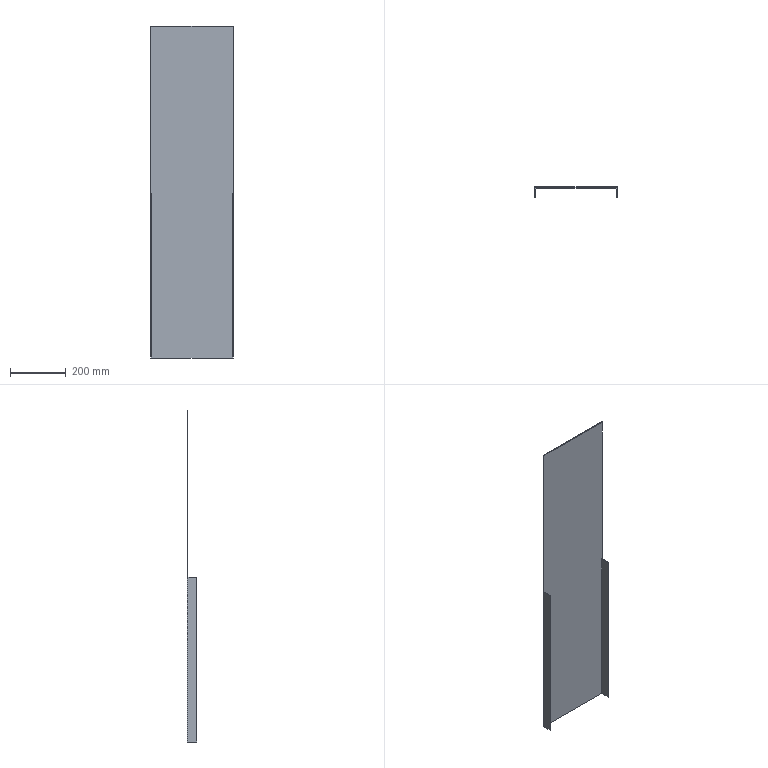Part | STEP file | Telescopic plate | 1 solid | 12 faces | box 296 x 35 x 1190 mm | volume 1170000 mm3 | plane 12
STEP:
#1=CARTESIAN_POINT('',(-41.136,41.939,1190.));
#2=VERTEX_POINT('',#1);
#3=CARTESIAN_POINT('',(-41.136,41.939,0.));
#4=VERTEX_POINT('',#3);
#5=CARTESIAN_POINT('',(-41.136,41.939,1190.));
#6=DIRECTION('',(0.,0.,-1.));
#7=VECTOR('',#6,1000.);
#8=LINE('',#5,#7);
#9=EDGE_CURVE('',#2,#4,#8,.T.);
#10=ORIENTED_EDGE('',*,*,#9,.F.);
#11=CARTESIAN_POINT('',(254.864,41.939,1190.));
#12=VERTEX_POINT('',#11);
#13=CARTESIAN_POINT('',(-41.136,41.939,1190.));
#14=DIRECTION('',(-1.,0.,0.));
#15=VECTOR('',#14,1000.);
#16=LINE('',#13,#15);
#17=EDGE_CURVE('',#12,#2,#16,.T.);
#18=ORIENTED_EDGE('',*,*,#17,.F.);
#19=CARTESIAN_POINT('',(254.864,41.939,0.));
#20=VERTEX_POINT('',#19);
#21=CARTESIAN_POINT('',(254.864,41.939,1190.));
#22=DIRECTION('',(0.,0.,1.));
#23=VECTOR('',#22,1000.);
#24=LINE('',#21,#23);
#25=EDGE_CURVE('',#20,#12,#24,.T.);
#26=ORIENTED_EDGE('',*,*,#25,.F.);
#27=CARTESIAN_POINT('',(-41.136,41.939,0.));
#28=DIRECTION('',(1.,0.,0.));
#29=VECTOR('',#28,1000.);
#30=LINE('',#27,#29);
#31=EDGE_CURVE('',#4,#20,#30,.T.);
#32=ORIENTED_EDGE('',*,*,#31,.F.);
#33=EDGE_LOOP('',(#10,#18,#26,#32));
#34=FACE_OUTER_BOUND('',#33,.T.);
#35=CARTESIAN_POINT('',(-41.136,41.939,1190.));
#36=DIRECTION('',(0.,-1.,0.));
#37=DIRECTION('',(0.,0.,-1.));
#38=AXIS2_PLACEMENT_3D('',#35,#36,#37);
#39=PLANE('',#38);
#40=ADVANCED_FACE('',(#34),#39,.F.);
#41=CARTESIAN_POINT('',(251.864,38.939,0.));
#42=VERTEX_POINT('',#41);
#43=CARTESIAN_POINT('',(-38.136,38.939,0.));
#44=VERTEX_POINT('',#43);
#45=CARTESIAN_POINT('',(-41.136,38.939,0.));
#46=DIRECTION('',(-1.,0.,0.));
#47=VECTOR('',#46,1000.);
#48=LINE('',#45,#47);
#49=EDGE_CURVE('',#42,#44,#48,.T.);
#50=ORIENTED_EDGE('',*,*,#49,.T.);
#51=CARTESIAN_POINT('',(-38.136,6.939,0.));
#52=VERTEX_POINT('',#51);
#53=CARTESIAN_POINT('',(-38.136,6.939,0.));
#54=DIRECTION('',(0.,-1.,0.));
#55=VECTOR('',#54,1000.);
#56=LINE('',#53,#55);
#57=EDGE_CURVE('',#44,#52,#56,.T.);
#58=ORIENTED_EDGE('',*,*,#57,.T.);
#59=CARTESIAN_POINT('',(-41.136,6.939,0.));
#60=VERTEX_POINT('',#59);
#61=CARTESIAN_POINT('',(-41.136,6.939,0.));
#62=DIRECTION('',(-1.,0.,0.));
#63=VECTOR('',#62,1000.);
#64=LINE('',#61,#63);
#65=EDGE_CURVE('',#52,#60,#64,.T.);
#66=ORIENTED_EDGE('',*,*,#65,.T.);
#67=CARTESIAN_POINT('',(-41.136,6.939,0.));
#68=DIRECTION('',(0.,1.,0.));
#69=VECTOR('',#68,1000.);
#70=LINE('',#67,#69);
#71=EDGE_CURVE('',#60,#4,#70,.T.);
#72=ORIENTED_EDGE('',*,*,#71,.T.);
#73=ORIENTED_EDGE('',*,*,#31,.T.);
#74=CARTESIAN_POINT('',(254.864,6.939,0.));
#75=VERTEX_POINT('',#74);
#76=CARTESIAN_POINT('',(254.864,6.939,0.));
#77=DIRECTION('',(0.,-1.,0.));
#78=VECTOR('',#77,1000.);
#79=LINE('',#76,#78);
#80=EDGE_CURVE('',#20,#75,#79,.T.);
#81=ORIENTED_EDGE('',*,*,#80,.T.);
#82=CARTESIAN_POINT('',(251.864,6.939,0.));
#83=VERTEX_POINT('',#82);
#84=CARTESIAN_POINT('',(-41.136,6.939,0.));
#85=DIRECTION('',(-1.,0.,0.));
#86=VECTOR('',#85,1000.);
#87=LINE('',#84,#86);
#88=EDGE_CURVE('',#75,#83,#87,.T.);
#89=ORIENTED_EDGE('',*,*,#88,.T.);
#90=CARTESIAN_POINT('',(251.864,6.939,0.));
#91=DIRECTION('',(0.,1.,0.));
#92=VECTOR('',#91,1000.);
#93=LINE('',#90,#92);
#94=EDGE_CURVE('',#83,#42,#93,.T.);
#95=ORIENTED_EDGE('',*,*,#94,.T.);
#96=EDGE_LOOP('',(#50,#58,#66,#72,#73,#81,#89,#95));
#97=FACE_OUTER_BOUND('',#96,.T.);
#98=CARTESIAN_POINT('',(-41.136,6.939,0.));
#99=DIRECTION('',(0.,0.,-1.));
#100=DIRECTION('',(-1.,0.,0.));
#101=AXIS2_PLACEMENT_3D('',#98,#99,#100);
#102=PLANE('',#101);
#103=ADVANCED_FACE('',(#97),#102,.T.);
#104=CARTESIAN_POINT('',(-41.136,38.939,1190.));
#105=VERTEX_POINT('',#104);
#106=CARTESIAN_POINT('',(-41.136,38.939,590.));
#107=VERTEX_POINT('',#106);
#108=CARTESIAN_POINT('',(-41.136,38.939,1190.));
#109=DIRECTION('',(0.,0.,-1.));
#110=VECTOR('',#109,1000.);
#111=LINE('',#108,#110);
#112=EDGE_CURVE('',#105,#107,#111,.T.);
#113=ORIENTED_EDGE('',*,*,#112,.F.);
#114=CARTESIAN_POINT('',(-41.136,6.939,1190.));
#115=DIRECTION('',(0.,-1.,0.));
#116=VECTOR('',#115,1000.);
#117=LINE('',#114,#116);
#118=EDGE_CURVE('',#2,#105,#117,.T.);
#119=ORIENTED_EDGE('',*,*,#118,.F.);
#120=ORIENTED_EDGE('',*,*,#9,.T.);
#121=ORIENTED_EDGE('',*,*,#71,.F.);
#122=CARTESIAN_POINT('',(-41.136,6.939,590.));
#123=VERTEX_POINT('',#122);
#124=CARTESIAN_POINT('',(-41.136,6.939,1190.));
#125=DIRECTION('',(0.,0.,-1.));
#126=VECTOR('',#125,1000.);
#127=LINE('',#124,#126);
#128=EDGE_CURVE('',#123,#60,#127,.T.);
#129=ORIENTED_EDGE('',*,*,#128,.F.);
#130=CARTESIAN_POINT('',(-41.136,6.939,590.));
#131=DIRECTION('',(0.,-1.,0.));
#132=VECTOR('',#131,1000.);
#133=LINE('',#130,#132);
#134=EDGE_CURVE('',#107,#123,#133,.T.);
#135=ORIENTED_EDGE('',*,*,#134,.F.);
#136=EDGE_LOOP('',(#113,#119,#120,#121,#129,#135));
#137=FACE_OUTER_BOUND('',#136,.T.);
#138=CARTESIAN_POINT('',(-41.136,6.939,1190.));
#139=DIRECTION('',(1.,0.,0.));
#140=DIRECTION('',(0.,0.,-1.));
#141=AXIS2_PLACEMENT_3D('',#138,#139,#140);
#142=PLANE('',#141);
#143=ADVANCED_FACE('',(#137),#142,.F.);
#144=CARTESIAN_POINT('',(254.864,38.939,1190.));
#145=VERTEX_POINT('',#144);
#146=CARTESIAN_POINT('',(-41.136,38.939,1190.));
#147=DIRECTION('',(-1.,0.,0.));
#148=VECTOR('',#147,1000.);
#149=LINE('',#146,#148);
#150=EDGE_CURVE('',#145,#105,#149,.T.);
#151=ORIENTED_EDGE('',*,*,#150,.F.);
#152=CARTESIAN_POINT('',(254.864,6.939,1190.));
#153=DIRECTION('',(0.,-1.,0.));
#154=VECTOR('',#153,1000.);
#155=LINE('',#152,#154);
#156=EDGE_CURVE('',#12,#145,#155,.T.);
#157=ORIENTED_EDGE('',*,*,#156,.F.);
#158=ORIENTED_EDGE('',*,*,#17,.T.);
#159=ORIENTED_EDGE('',*,*,#118,.T.);
#160=EDGE_LOOP('',(#151,#157,#158,#159));
#161=FACE_OUTER_BOUND('',#160,.T.);
#162=CARTESIAN_POINT('',(-41.136,6.939,1190.));
#163=DIRECTION('',(0.,0.,-1.));
#164=DIRECTION('',(-1.,0.,0.));
#165=AXIS2_PLACEMENT_3D('',#162,#163,#164);
#166=PLANE('',#165);
#167=ADVANCED_FACE('',(#161),#166,.F.);
#168=CARTESIAN_POINT('',(254.864,38.939,590.));
#169=VERTEX_POINT('',#168);
#170=CARTESIAN_POINT('',(254.864,38.939,1190.));
#171=DIRECTION('',(0.,0.,1.));
#172=VECTOR('',#171,1000.);
#173=LINE('',#170,#172);
#174=EDGE_CURVE('',#169,#145,#173,.T.);
#175=ORIENTED_EDGE('',*,*,#174,.F.);
#176=CARTESIAN_POINT('',(254.864,6.939,590.));
#177=VERTEX_POINT('',#176);
#178=CARTESIAN_POINT('',(254.864,41.939,590.));
#179=DIRECTION('',(0.,1.,0.));
#180=VECTOR('',#179,1000.);
#181=LINE('',#178,#180);
#182=EDGE_CURVE('',#177,#169,#181,.T.);
#183=ORIENTED_EDGE('',*,*,#182,.F.);
#184=CARTESIAN_POINT('',(254.864,6.939,1190.));
#185=DIRECTION('',(0.,0.,1.));
#186=VECTOR('',#185,1000.);
#187=LINE('',#184,#186);
#188=EDGE_CURVE('',#75,#177,#187,.T.);
#189=ORIENTED_EDGE('',*,*,#188,.F.);
#190=ORIENTED_EDGE('',*,*,#80,.F.);
#191=ORIENTED_EDGE('',*,*,#25,.T.);
#192=ORIENTED_EDGE('',*,*,#156,.T.);
#193=EDGE_LOOP('',(#175,#183,#189,#190,#191,#192));
#194=FACE_OUTER_BOUND('',#193,.T.);
#195=CARTESIAN_POINT('',(254.864,41.939,1190.));
#196=DIRECTION('',(-1.,0.,0.));
#197=DIRECTION('',(0.,0.,1.));
#198=AXIS2_PLACEMENT_3D('',#195,#196,#197);
#199=PLANE('',#198);
#200=ADVANCED_FACE('',(#194),#199,.F.);
#201=CARTESIAN_POINT('',(-38.136,6.939,590.));
#202=VERTEX_POINT('',#201);
#203=CARTESIAN_POINT('',(-38.136,38.939,590.));
#204=VERTEX_POINT('',#203);
#205=CARTESIAN_POINT('',(-38.136,6.939,590.));
#206=DIRECTION('',(0.,1.,0.));
#207=VECTOR('',#206,1000.);
#208=LINE('',#205,#207);
#209=EDGE_CURVE('',#202,#204,#208,.T.);
#210=ORIENTED_EDGE('',*,*,#209,.F.);
#211=CARTESIAN_POINT('',(-38.136,6.939,1190.));
#212=DIRECTION('',(0.,0.,1.));
#213=VECTOR('',#212,1000.);
#214=LINE('',#211,#213);
#215=EDGE_CURVE('',#52,#202,#214,.T.);
#216=ORIENTED_EDGE('',*,*,#215,.F.);
#217=ORIENTED_EDGE('',*,*,#57,.F.);
#218=CARTESIAN_POINT('',(-38.136,38.939,1190.));
#219=DIRECTION('',(0.,0.,-1.));
#220=VECTOR('',#219,1000.);
#221=LINE('',#218,#220);
#222=EDGE_CURVE('',#204,#44,#221,.T.);
#223=ORIENTED_EDGE('',*,*,#222,.F.);
#224=EDGE_LOOP('',(#210,#216,#217,#223));
#225=FACE_OUTER_BOUND('',#224,.T.);
#226=CARTESIAN_POINT('',(-38.136,6.939,1190.));
#227=DIRECTION('',(-1.,0.,0.));
#228=DIRECTION('',(0.,0.,1.));
#229=AXIS2_PLACEMENT_3D('',#226,#227,#228);
#230=PLANE('',#229);
#231=ADVANCED_FACE('',(#225),#230,.F.);
#232=CARTESIAN_POINT('',(251.864,38.939,590.));
#233=VERTEX_POINT('',#232);
#234=CARTESIAN_POINT('',(-38.136,38.939,590.));
#235=DIRECTION('',(-1.,0.,0.));
#236=VECTOR('',#235,1000.);
#237=LINE('',#234,#236);
#238=EDGE_CURVE('',#169,#233,#237,.T.);
#239=ORIENTED_EDGE('',*,*,#238,.F.);
#240=ORIENTED_EDGE('',*,*,#174,.T.);
#241=ORIENTED_EDGE('',*,*,#150,.T.);
#242=ORIENTED_EDGE('',*,*,#112,.T.);
#243=CARTESIAN_POINT('',(-38.136,38.939,590.));
#244=DIRECTION('',(-1.,0.,0.));
#245=VECTOR('',#244,1000.);
#246=LINE('',#243,#245);
#247=EDGE_CURVE('',#204,#107,#246,.T.);
#248=ORIENTED_EDGE('',*,*,#247,.F.);
#249=ORIENTED_EDGE('',*,*,#222,.T.);
#250=ORIENTED_EDGE('',*,*,#49,.F.);
#251=CARTESIAN_POINT('',(251.864,38.939,1190.));
#252=DIRECTION('',(0.,0.,-1.));
#253=VECTOR('',#252,1000.);
#254=LINE('',#251,#253);
#255=EDGE_CURVE('',#233,#42,#254,.T.);
#256=ORIENTED_EDGE('',*,*,#255,.F.);
#257=EDGE_LOOP('',(#239,#240,#241,#242,#248,#249,#250,#256));
#258=FACE_OUTER_BOUND('',#257,.T.);
#259=CARTESIAN_POINT('',(-38.136,38.939,1190.));
#260=DIRECTION('',(0.,1.,0.));
#261=DIRECTION('',(0.,0.,1.));
#262=AXIS2_PLACEMENT_3D('',#259,#260,#261);
#263=PLANE('',#262);
#264=ADVANCED_FACE('',(#258),#263,.F.);
#265=CARTESIAN_POINT('',(251.864,6.939,590.));
#266=VERTEX_POINT('',#265);
#267=CARTESIAN_POINT('',(251.864,38.939,590.));
#268=DIRECTION('',(0.,-1.,0.));
#269=VECTOR('',#268,1000.);
#270=LINE('',#267,#269);
#271=EDGE_CURVE('',#233,#266,#270,.T.);
#272=ORIENTED_EDGE('',*,*,#271,.F.);
#273=ORIENTED_EDGE('',*,*,#255,.T.);
#274=ORIENTED_EDGE('',*,*,#94,.F.);
#275=CARTESIAN_POINT('',(251.864,6.939,1190.));
#276=DIRECTION('',(0.,0.,-1.));
#277=VECTOR('',#276,1000.);
#278=LINE('',#275,#277);
#279=EDGE_CURVE('',#266,#83,#278,.T.);
#280=ORIENTED_EDGE('',*,*,#279,.F.);
#281=EDGE_LOOP('',(#272,#273,#274,#280));
#282=FACE_OUTER_BOUND('',#281,.T.);
#283=CARTESIAN_POINT('',(251.864,38.939,1190.));
#284=DIRECTION('',(1.,0.,0.));
#285=DIRECTION('',(0.,0.,-1.));
#286=AXIS2_PLACEMENT_3D('',#283,#284,#285);
#287=PLANE('',#286);
#288=ADVANCED_FACE('',(#282),#287,.F.);
#289=CARTESIAN_POINT('',(251.864,6.939,590.));
#290=DIRECTION('',(1.,0.,0.));
#291=VECTOR('',#290,1000.);
#292=LINE('',#289,#291);
#293=EDGE_CURVE('',#266,#177,#292,.T.);
#294=ORIENTED_EDGE('',*,*,#293,.F.);
#295=ORIENTED_EDGE('',*,*,#279,.T.);
#296=ORIENTED_EDGE('',*,*,#88,.F.);
#297=ORIENTED_EDGE('',*,*,#188,.T.);
#298=EDGE_LOOP('',(#294,#295,#296,#297));
#299=FACE_OUTER_BOUND('',#298,.T.);
#300=CARTESIAN_POINT('',(251.864,6.939,1190.));
#301=DIRECTION('',(0.,1.,0.));
#302=DIRECTION('',(0.,0.,1.));
#303=AXIS2_PLACEMENT_3D('',#300,#301,#302);
#304=PLANE('',#303);
#305=ADVANCED_FACE('',(#299),#304,.F.);
#306=CARTESIAN_POINT('',(-38.136,6.939,590.));
#307=DIRECTION('',(1.,0.,0.));
#308=VECTOR('',#307,1000.);
#309=LINE('',#306,#308);
#310=EDGE_CURVE('',#123,#202,#309,.T.);
#311=ORIENTED_EDGE('',*,*,#310,.F.);
#312=ORIENTED_EDGE('',*,*,#128,.T.);
#313=ORIENTED_EDGE('',*,*,#65,.F.);
#314=ORIENTED_EDGE('',*,*,#215,.T.);
#315=EDGE_LOOP('',(#311,#312,#313,#314));
#316=FACE_OUTER_BOUND('',#315,.T.);
#317=CARTESIAN_POINT('',(-38.136,6.939,1190.));
#318=DIRECTION('',(0.,1.,0.));
#319=DIRECTION('',(0.,0.,1.));
#320=AXIS2_PLACEMENT_3D('',#317,#318,#319);
#321=PLANE('',#320);
#322=ADVANCED_FACE('',(#316),#321,.F.);
#323=ORIENTED_EDGE('',*,*,#134,.T.);
#324=ORIENTED_EDGE('',*,*,#310,.T.);
#325=ORIENTED_EDGE('',*,*,#209,.T.);
#326=ORIENTED_EDGE('',*,*,#247,.T.);
#327=EDGE_LOOP('',(#323,#324,#325,#326));
#328=FACE_OUTER_BOUND('',#327,.T.);
#329=CARTESIAN_POINT('',(-135.136,6.939,590.));
#330=DIRECTION('',(0.,0.,-1.));
#331=DIRECTION('',(-1.,0.,0.));
#332=AXIS2_PLACEMENT_3D('',#329,#330,#331);
#333=PLANE('',#332);
#334=ADVANCED_FACE('',(#328),#333,.F.);
#335=ORIENTED_EDGE('',*,*,#182,.T.);
#336=ORIENTED_EDGE('',*,*,#238,.T.);
#337=ORIENTED_EDGE('',*,*,#271,.T.);
#338=ORIENTED_EDGE('',*,*,#293,.T.);
#339=EDGE_LOOP('',(#335,#336,#337,#338));
#340=FACE_OUTER_BOUND('',#339,.T.);
#341=CARTESIAN_POINT('',(-135.136,6.939,590.));
#342=DIRECTION('',(0.,0.,-1.));
#343=DIRECTION('',(-1.,0.,0.));
#344=AXIS2_PLACEMENT_3D('',#341,#342,#343);
#345=PLANE('',#344);
#346=ADVANCED_FACE('',(#340),#345,.F.);
#347=CLOSED_SHELL('',(#40,#103,#143,#167,#200,#231,#264,#288,#305,#322,#334,#346));
#348=MANIFOLD_SOLID_BREP('',#347);
#349=CARTESIAN_POINT('',(0.,0.,0.));
#350=DIRECTION('',(0.,0.,1.));
#351=DIRECTION('',(1.,0.,0.));
#352=AXIS2_PLACEMENT_3D('',#349,#350,#351);
#353=(LENGTH_UNIT()NAMED_UNIT(*)SI_UNIT(.MILLI.,.METRE.));
#354=UNCERTAINTY_MEASURE_WITH_UNIT(LENGTH_MEASURE(0.00001),#353,'','');
#355=(NAMED_UNIT(*)PLANE_ANGLE_UNIT()SI_UNIT($,.RADIAN.));
#356=(NAMED_UNIT(*)SI_UNIT($,.STERADIAN.)SOLID_ANGLE_UNIT());
#357=(GEOMETRIC_REPRESENTATION_CONTEXT(3)GLOBAL_UNCERTAINTY_ASSIGNED_CONTEXT((#354))GLOBAL_UNIT_ASSIGNED_CONTEXT((#353,#355,#356))REPRESENTATION_CONTEXT('',''));
#358=ADVANCED_BREP_SHAPE_REPRESENTATION('',(#348,#352),#357);